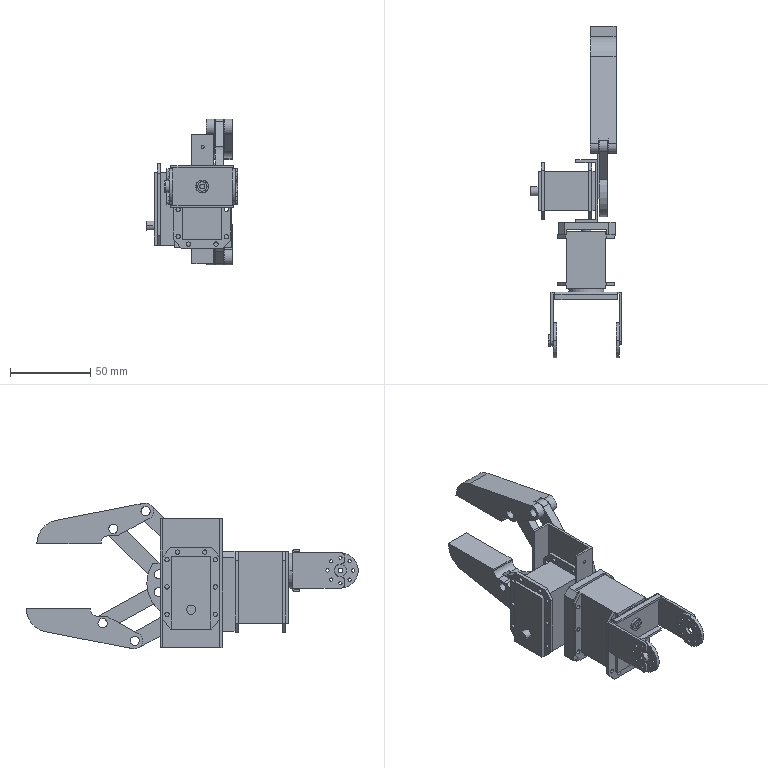Part | SolidWorks | 15 solids | 469 faces | box 56.883 x 206.393 x 90.637 mm | volume 149164 mm3 | cylinder 283 | plane 186 | commonest cylinder face diameters 2 x78 2.7 x76 5.7 x50 10 x14 8 x10 4 x8